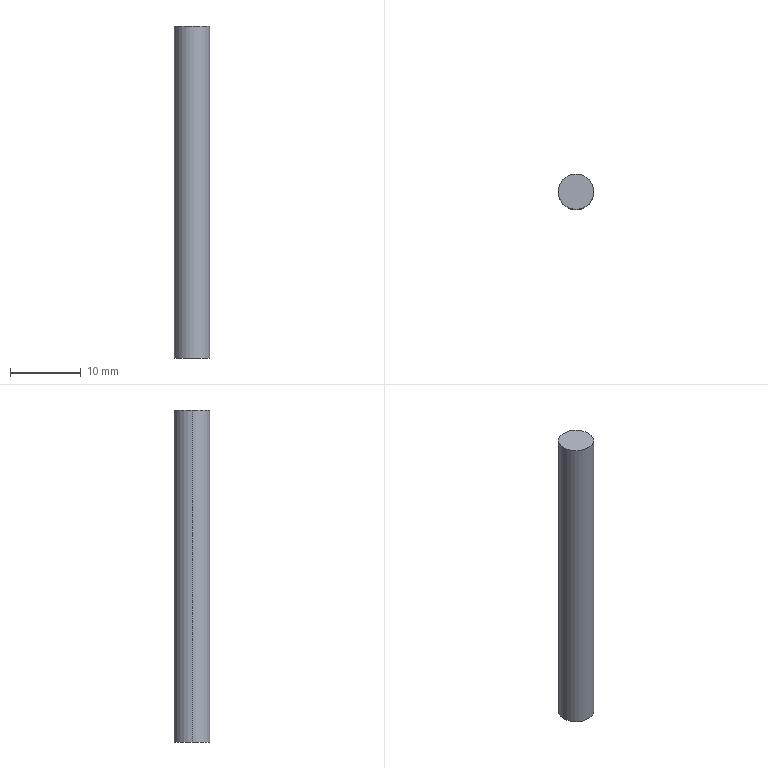Part | NX | features BREP 1 | 1 solid | 4 faces | box 5 x 5 x 47 mm | volume 922.843 mm3 | cylinder 2 | plane 2 | commonest cylinder face diameters 5 x2
STEP:
#1=CARTESIAN_POINT('',(2.5,0.,47.));
#2=VERTEX_POINT('',#1);
#3=CARTESIAN_POINT('',(-2.5,0.,47.));
#4=VERTEX_POINT('',#3);
#5=CARTESIAN_POINT('',(0.,0.,47.));
#6=DIRECTION('',(0.,0.,1.));
#7=DIRECTION('',(1.,0.,0.));
#8=AXIS2_PLACEMENT_3D('',#5,#6,#7);
#9=CIRCLE('',#8,2.5);
#10=EDGE_CURVE('',#2,#4,#9,.T.);
#11=ORIENTED_EDGE('',*,*,#10,.F.);
#12=CARTESIAN_POINT('',(2.5,0.,0.));
#13=VERTEX_POINT('',#12);
#14=CARTESIAN_POINT('',(2.5,0.,47.));
#15=DIRECTION('',(0.,0.,-1.));
#16=VECTOR('',#15,1000.);
#17=LINE('',#14,#16);
#18=EDGE_CURVE('',#2,#13,#17,.T.);
#19=ORIENTED_EDGE('',*,*,#18,.T.);
#20=CARTESIAN_POINT('',(-2.5,0.,0.));
#21=VERTEX_POINT('',#20);
#22=CARTESIAN_POINT('',(0.,0.,0.));
#23=DIRECTION('',(0.,0.,1.));
#24=DIRECTION('',(1.,0.,0.));
#25=AXIS2_PLACEMENT_3D('',#22,#23,#24);
#26=CIRCLE('',#25,2.5);
#27=EDGE_CURVE('',#13,#21,#26,.T.);
#28=ORIENTED_EDGE('',*,*,#27,.T.);
#29=CARTESIAN_POINT('',(-2.5,0.,47.));
#30=DIRECTION('',(0.,0.,-1.));
#31=VECTOR('',#30,1000.);
#32=LINE('',#29,#31);
#33=EDGE_CURVE('',#4,#21,#32,.T.);
#34=ORIENTED_EDGE('',*,*,#33,.F.);
#35=EDGE_LOOP('',(#11,#19,#28,#34));
#36=FACE_BOUND('',#35,.T.);
#37=CARTESIAN_POINT('',(0.,0.,47.));
#38=DIRECTION('',(0.,0.,-1.));
#39=DIRECTION('',(-1.,0.,0.));
#40=AXIS2_PLACEMENT_3D('',#37,#38,#39);
#41=CYLINDRICAL_SURFACE('',#40,2.5);
#42=ADVANCED_FACE('',(#36),#41,.T.);
#43=ORIENTED_EDGE('',*,*,#18,.F.);
#44=CARTESIAN_POINT('',(0.,0.,47.));
#45=DIRECTION('',(0.,0.,1.));
#46=DIRECTION('',(1.,0.,0.));
#47=AXIS2_PLACEMENT_3D('',#44,#45,#46);
#48=CIRCLE('',#47,2.5);
#49=EDGE_CURVE('',#4,#2,#48,.T.);
#50=ORIENTED_EDGE('',*,*,#49,.F.);
#51=ORIENTED_EDGE('',*,*,#33,.T.);
#52=CARTESIAN_POINT('',(0.,0.,0.));
#53=DIRECTION('',(0.,0.,1.));
#54=DIRECTION('',(1.,0.,0.));
#55=AXIS2_PLACEMENT_3D('',#52,#53,#54);
#56=CIRCLE('',#55,2.5);
#57=EDGE_CURVE('',#21,#13,#56,.T.);
#58=ORIENTED_EDGE('',*,*,#57,.T.);
#59=EDGE_LOOP('',(#43,#50,#51,#58));
#60=FACE_BOUND('',#59,.T.);
#61=CARTESIAN_POINT('',(0.,0.,47.));
#62=DIRECTION('',(0.,0.,-1.));
#63=DIRECTION('',(-1.,0.,0.));
#64=AXIS2_PLACEMENT_3D('',#61,#62,#63);
#65=CYLINDRICAL_SURFACE('',#64,2.5);
#66=ADVANCED_FACE('',(#60),#65,.T.);
#67=ORIENTED_EDGE('',*,*,#49,.T.);
#68=ORIENTED_EDGE('',*,*,#10,.T.);
#69=EDGE_LOOP('',(#67,#68));
#70=FACE_BOUND('',#69,.T.);
#71=CARTESIAN_POINT('',(0.,0.,47.));
#72=DIRECTION('',(0.,0.,1.));
#73=DIRECTION('',(1.,0.,0.));
#74=AXIS2_PLACEMENT_3D('',#71,#72,#73);
#75=PLANE('',#74);
#76=ADVANCED_FACE('',(#70),#75,.T.);
#77=ORIENTED_EDGE('',*,*,#57,.F.);
#78=ORIENTED_EDGE('',*,*,#27,.F.);
#79=EDGE_LOOP('',(#77,#78));
#80=FACE_BOUND('',#79,.T.);
#81=CARTESIAN_POINT('',(0.,0.,0.));
#82=DIRECTION('',(0.,0.,1.));
#83=DIRECTION('',(1.,0.,0.));
#84=AXIS2_PLACEMENT_3D('',#81,#82,#83);
#85=PLANE('',#84);
#86=ADVANCED_FACE('',(#80),#85,.F.);
#87=CLOSED_SHELL('',(#42,#66,#76,#86));
#88=MANIFOLD_SOLID_BREP('',#87);
#89=(LENGTH_UNIT()NAMED_UNIT(*)SI_UNIT(.MILLI.,.METRE.));
#90=UNCERTAINTY_MEASURE_WITH_UNIT(LENGTH_MEASURE(0.00001),#89,'','');
#91=(NAMED_UNIT(*)PLANE_ANGLE_UNIT()SI_UNIT($,.RADIAN.));
#92=(NAMED_UNIT(*)SI_UNIT($,.STERADIAN.)SOLID_ANGLE_UNIT());
#93=(GEOMETRIC_REPRESENTATION_CONTEXT(3)GLOBAL_UNCERTAINTY_ASSIGNED_CONTEXT((#90))GLOBAL_UNIT_ASSIGNED_CONTEXT((#89,#91,#92))REPRESENTATION_CONTEXT('',''));
#94=ADVANCED_BREP_SHAPE_REPRESENTATION('',(#88),#93);